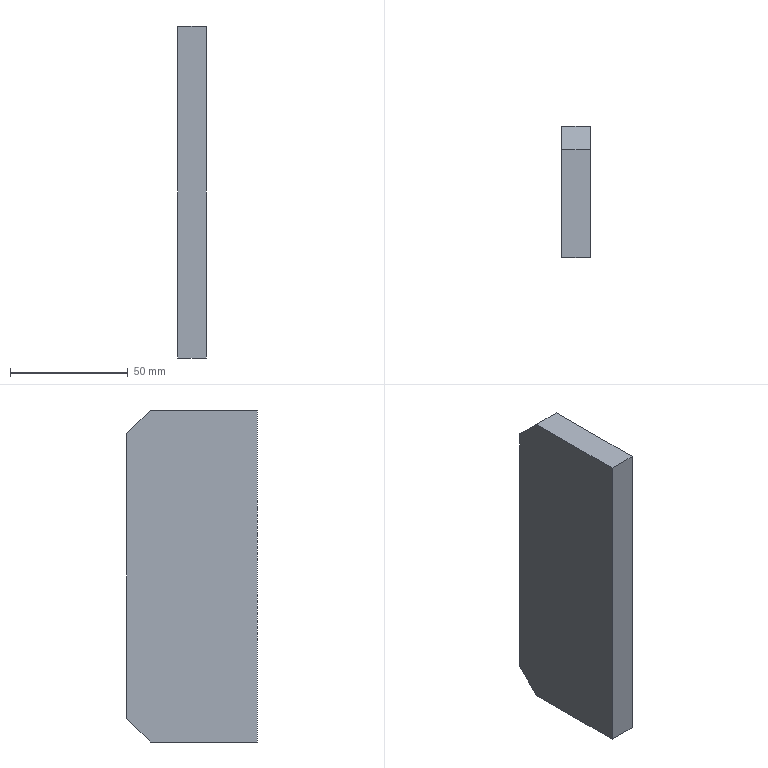Part | STEP file | RIB.1.stp | 1 solid | 8 faces | box 12 x 55.5 x 141 mm | volume 92706 mm3 | plane 8
STEP:
#1=CARTESIAN_POINT('',(0.,0.,0.));
#2=DIRECTION('',(0.,0.,1.));
#3=DIRECTION('',(1.,0.,0.));
#4=AXIS2_PLACEMENT_3D('',#1,#2,#3);
#5=CARTESIAN_POINT('',(6.,-27.75,-70.5));
#6=VERTEX_POINT('',#5);
#7=CARTESIAN_POINT('',(6.,17.75,-70.5));
#8=VERTEX_POINT('',#7);
#9=CARTESIAN_POINT('',(6.,-27.75,-70.5));
#10=DIRECTION('',(0.,1.,0.));
#11=VECTOR('',#10,1.);
#12=LINE('',#9,#11);
#13=CARTESIAN_POINT('',(6.,-0.9613,0.));
#14=DIRECTION('',(1.,0.,0.));
#15=DIRECTION('',(0.,1.,0.));
#16=AXIS2_PLACEMENT_3D('',#13,#14,#15);
#17=PLANE('',#16);
#18=CARTESIAN_POINT('',(-26.789,-70.5));
#19=DIRECTION('',(1.,0.));
#20=VECTOR('',#19,1.);
#21=LINE('',#18,#20);
#22=(GEOMETRIC_REPRESENTATION_CONTEXT(2)PARAMETRIC_REPRESENTATION_CONTEXT()REPRESENTATION_CONTEXT('',''));
#23=DEFINITIONAL_REPRESENTATION('',(#21),#22);
#24=PCURVE('',#17,#23);
#25=CARTESIAN_POINT('',(6.,-27.75,-70.5));
#26=DIRECTION('',(0.,0.,-1.));
#27=DIRECTION('',(0.,-1.,0.));
#28=AXIS2_PLACEMENT_3D('',#25,#26,#27);
#29=PLANE('',#28);
#30=CARTESIAN_POINT('',(0.,0.));
#31=DIRECTION('',(-1.,0.));
#32=VECTOR('',#31,1.);
#33=LINE('',#30,#32);
#34=(GEOMETRIC_REPRESENTATION_CONTEXT(2)PARAMETRIC_REPRESENTATION_CONTEXT()REPRESENTATION_CONTEXT('',''));
#35=DEFINITIONAL_REPRESENTATION('',(#33),#34);
#36=PCURVE('',#29,#35);
#37=SURFACE_CURVE('',#12,(#24,#36),.PCURVE_S1.);
#38=EDGE_CURVE('',#6,#8,#37,.T.);
#39=ORIENTED_EDGE('',*,*,#38,.T.);
#40=CARTESIAN_POINT('',(6.,27.75,-60.5));
#41=VERTEX_POINT('',#40);
#42=CARTESIAN_POINT('',(6.,17.75,-70.5));
#43=DIRECTION('',(0.,0.7071,0.7071));
#44=VECTOR('',#43,1.);
#45=LINE('',#42,#44);
#46=CARTESIAN_POINT('',(18.711,-70.5));
#47=DIRECTION('',(0.7071,0.7071));
#48=VECTOR('',#47,1.);
#49=LINE('',#46,#48);
#50=(GEOMETRIC_REPRESENTATION_CONTEXT(2)PARAMETRIC_REPRESENTATION_CONTEXT()REPRESENTATION_CONTEXT('',''));
#51=DEFINITIONAL_REPRESENTATION('',(#49),#50);
#52=PCURVE('',#17,#51);
#53=CARTESIAN_POINT('',(6.,17.75,-70.5));
#54=DIRECTION('',(0.,0.7071,-0.7071));
#55=DIRECTION('',(-1.,0.,0.));
#56=AXIS2_PLACEMENT_3D('',#53,#54,#55);
#57=PLANE('',#56);
#58=CARTESIAN_POINT('',(0.,0.));
#59=DIRECTION('',(0.,1.));
#60=VECTOR('',#59,1.);
#61=LINE('',#58,#60);
#62=(GEOMETRIC_REPRESENTATION_CONTEXT(2)PARAMETRIC_REPRESENTATION_CONTEXT()REPRESENTATION_CONTEXT('',''));
#63=DEFINITIONAL_REPRESENTATION('',(#61),#62);
#64=PCURVE('',#57,#63);
#65=SURFACE_CURVE('',#45,(#52,#64),.PCURVE_S1.);
#66=EDGE_CURVE('',#8,#41,#65,.T.);
#67=ORIENTED_EDGE('',*,*,#66,.T.);
#68=CARTESIAN_POINT('',(6.,27.75,60.5));
#69=VERTEX_POINT('',#68);
#70=CARTESIAN_POINT('',(6.,27.75,-60.5));
#71=DIRECTION('',(0.,0.,1.));
#72=VECTOR('',#71,1.);
#73=LINE('',#70,#72);
#74=CARTESIAN_POINT('',(28.711,-60.5));
#75=DIRECTION('',(0.,1.));
#76=VECTOR('',#75,1.);
#77=LINE('',#74,#76);
#78=(GEOMETRIC_REPRESENTATION_CONTEXT(2)PARAMETRIC_REPRESENTATION_CONTEXT()REPRESENTATION_CONTEXT('',''));
#79=DEFINITIONAL_REPRESENTATION('',(#77),#78);
#80=PCURVE('',#17,#79);
#81=CARTESIAN_POINT('',(6.,27.75,-60.5));
#82=DIRECTION('',(0.,1.,0.));
#83=DIRECTION('',(1.,0.,0.));
#84=AXIS2_PLACEMENT_3D('',#81,#82,#83);
#85=PLANE('',#84);
#86=CARTESIAN_POINT('',(0.,0.));
#87=DIRECTION('',(0.,-1.));
#88=VECTOR('',#87,1.);
#89=LINE('',#86,#88);
#90=(GEOMETRIC_REPRESENTATION_CONTEXT(2)PARAMETRIC_REPRESENTATION_CONTEXT()REPRESENTATION_CONTEXT('',''));
#91=DEFINITIONAL_REPRESENTATION('',(#89),#90);
#92=PCURVE('',#85,#91);
#93=SURFACE_CURVE('',#73,(#80,#92),.PCURVE_S1.);
#94=EDGE_CURVE('',#41,#69,#93,.T.);
#95=ORIENTED_EDGE('',*,*,#94,.T.);
#96=CARTESIAN_POINT('',(6.,17.75,70.5));
#97=VERTEX_POINT('',#96);
#98=CARTESIAN_POINT('',(6.,27.75,60.5));
#99=DIRECTION('',(0.,-0.7071,0.7071));
#100=VECTOR('',#99,1.);
#101=LINE('',#98,#100);
#102=CARTESIAN_POINT('',(28.711,60.5));
#103=DIRECTION('',(-0.7071,0.7071));
#104=VECTOR('',#103,1.);
#105=LINE('',#102,#104);
#106=(GEOMETRIC_REPRESENTATION_CONTEXT(2)PARAMETRIC_REPRESENTATION_CONTEXT()REPRESENTATION_CONTEXT('',''));
#107=DEFINITIONAL_REPRESENTATION('',(#105),#106);
#108=PCURVE('',#17,#107);
#109=CARTESIAN_POINT('',(6.,27.75,60.5));
#110=DIRECTION('',(0.,0.7071,0.7071));
#111=DIRECTION('',(1.,0.,0.));
#112=AXIS2_PLACEMENT_3D('',#109,#110,#111);
#113=PLANE('',#112);
#114=CARTESIAN_POINT('',(0.,0.));
#115=DIRECTION('',(0.,-1.));
#116=VECTOR('',#115,1.);
#117=LINE('',#114,#116);
#118=(GEOMETRIC_REPRESENTATION_CONTEXT(2)PARAMETRIC_REPRESENTATION_CONTEXT()REPRESENTATION_CONTEXT('',''));
#119=DEFINITIONAL_REPRESENTATION('',(#117),#118);
#120=PCURVE('',#113,#119);
#121=SURFACE_CURVE('',#101,(#108,#120),.PCURVE_S1.);
#122=EDGE_CURVE('',#69,#97,#121,.T.);
#123=ORIENTED_EDGE('',*,*,#122,.T.);
#124=CARTESIAN_POINT('',(6.,-27.75,70.5));
#125=VERTEX_POINT('',#124);
#126=CARTESIAN_POINT('',(6.,17.75,70.5));
#127=DIRECTION('',(0.,-1.,0.));
#128=VECTOR('',#127,1.);
#129=LINE('',#126,#128);
#130=CARTESIAN_POINT('',(18.711,70.5));
#131=DIRECTION('',(-1.,0.));
#132=VECTOR('',#131,1.);
#133=LINE('',#130,#132);
#134=(GEOMETRIC_REPRESENTATION_CONTEXT(2)PARAMETRIC_REPRESENTATION_CONTEXT()REPRESENTATION_CONTEXT('',''));
#135=DEFINITIONAL_REPRESENTATION('',(#133),#134);
#136=PCURVE('',#17,#135);
#137=CARTESIAN_POINT('',(6.,17.75,70.5));
#138=DIRECTION('',(0.,0.,1.));
#139=DIRECTION('',(1.,0.,0.));
#140=AXIS2_PLACEMENT_3D('',#137,#138,#139);
#141=PLANE('',#140);
#142=CARTESIAN_POINT('',(0.,0.));
#143=DIRECTION('',(0.,-1.));
#144=VECTOR('',#143,1.);
#145=LINE('',#142,#144);
#146=(GEOMETRIC_REPRESENTATION_CONTEXT(2)PARAMETRIC_REPRESENTATION_CONTEXT()REPRESENTATION_CONTEXT('',''));
#147=DEFINITIONAL_REPRESENTATION('',(#145),#146);
#148=PCURVE('',#141,#147);
#149=SURFACE_CURVE('',#129,(#136,#148),.PCURVE_S1.);
#150=EDGE_CURVE('',#97,#125,#149,.T.);
#151=ORIENTED_EDGE('',*,*,#150,.T.);
#152=CARTESIAN_POINT('',(6.,-27.75,-70.5));
#153=DIRECTION('',(0.,0.,1.));
#154=VECTOR('',#153,1.);
#155=LINE('',#152,#154);
#156=CARTESIAN_POINT('',(-26.789,-70.5));
#157=DIRECTION('',(0.,1.));
#158=VECTOR('',#157,1.);
#159=LINE('',#156,#158);
#160=(GEOMETRIC_REPRESENTATION_CONTEXT(2)PARAMETRIC_REPRESENTATION_CONTEXT()REPRESENTATION_CONTEXT('',''));
#161=DEFINITIONAL_REPRESENTATION('',(#159),#160);
#162=PCURVE('',#17,#161);
#163=CARTESIAN_POINT('',(6.,-27.75,70.5));
#164=DIRECTION('',(0.,-1.,0.));
#165=DIRECTION('',(0.,0.,-1.));
#166=AXIS2_PLACEMENT_3D('',#163,#164,#165);
#167=PLANE('',#166);
#168=CARTESIAN_POINT('',(141.,0.));
#169=DIRECTION('',(-1.,0.));
#170=VECTOR('',#169,1.);
#171=LINE('',#168,#170);
#172=(GEOMETRIC_REPRESENTATION_CONTEXT(2)PARAMETRIC_REPRESENTATION_CONTEXT()REPRESENTATION_CONTEXT('',''));
#173=DEFINITIONAL_REPRESENTATION('',(#171),#172);
#174=PCURVE('',#167,#173);
#175=SURFACE_CURVE('',#155,(#162,#174),.PCURVE_S1.);
#176=EDGE_CURVE('',#6,#125,#175,.T.);
#177=ORIENTED_EDGE('',*,*,#176,.F.);
#178=EDGE_LOOP('',(#39,#67,#95,#123,#151,#177));
#179=FACE_BOUND('',#178,.T.);
#180=ADVANCED_FACE('',(#179),#17,.T.);
#181=CARTESIAN_POINT('',(-6.,17.75,-70.5));
#182=VERTEX_POINT('',#181);
#183=CARTESIAN_POINT('',(-6.,27.75,-60.5));
#184=VERTEX_POINT('',#183);
#185=CARTESIAN_POINT('',(-6.,17.75,-70.5));
#186=DIRECTION('',(0.,0.7071,0.7071));
#187=VECTOR('',#186,1.);
#188=LINE('',#185,#187);
#189=CARTESIAN_POINT('',(-6.,-0.9613,0.));
#190=DIRECTION('',(1.,0.,0.));
#191=DIRECTION('',(0.,1.,0.));
#192=AXIS2_PLACEMENT_3D('',#189,#190,#191);
#193=PLANE('',#192);
#194=CARTESIAN_POINT('',(18.711,-70.5));
#195=DIRECTION('',(0.7071,0.7071));
#196=VECTOR('',#195,1.);
#197=LINE('',#194,#196);
#198=(GEOMETRIC_REPRESENTATION_CONTEXT(2)PARAMETRIC_REPRESENTATION_CONTEXT()REPRESENTATION_CONTEXT('',''));
#199=DEFINITIONAL_REPRESENTATION('',(#197),#198);
#200=PCURVE('',#193,#199);
#201=CARTESIAN_POINT('',(12.,0.));
#202=DIRECTION('',(0.,1.));
#203=VECTOR('',#202,1.);
#204=LINE('',#201,#203);
#205=(GEOMETRIC_REPRESENTATION_CONTEXT(2)PARAMETRIC_REPRESENTATION_CONTEXT()REPRESENTATION_CONTEXT('',''));
#206=DEFINITIONAL_REPRESENTATION('',(#204),#205);
#207=PCURVE('',#57,#206);
#208=SURFACE_CURVE('',#188,(#200,#207),.PCURVE_S1.);
#209=EDGE_CURVE('',#182,#184,#208,.T.);
#210=ORIENTED_EDGE('',*,*,#209,.F.);
#211=CARTESIAN_POINT('',(-6.,-27.75,-70.5));
#212=VERTEX_POINT('',#211);
#213=CARTESIAN_POINT('',(-6.,-27.75,-70.5));
#214=DIRECTION('',(0.,1.,0.));
#215=VECTOR('',#214,1.);
#216=LINE('',#213,#215);
#217=CARTESIAN_POINT('',(-26.789,-70.5));
#218=DIRECTION('',(1.,0.));
#219=VECTOR('',#218,1.);
#220=LINE('',#217,#219);
#221=(GEOMETRIC_REPRESENTATION_CONTEXT(2)PARAMETRIC_REPRESENTATION_CONTEXT()REPRESENTATION_CONTEXT('',''));
#222=DEFINITIONAL_REPRESENTATION('',(#220),#221);
#223=PCURVE('',#193,#222);
#224=CARTESIAN_POINT('',(0.,12.));
#225=DIRECTION('',(-1.,0.));
#226=VECTOR('',#225,1.);
#227=LINE('',#224,#226);
#228=(GEOMETRIC_REPRESENTATION_CONTEXT(2)PARAMETRIC_REPRESENTATION_CONTEXT()REPRESENTATION_CONTEXT('',''));
#229=DEFINITIONAL_REPRESENTATION('',(#227),#228);
#230=PCURVE('',#29,#229);
#231=SURFACE_CURVE('',#216,(#223,#230),.PCURVE_S1.);
#232=EDGE_CURVE('',#212,#182,#231,.T.);
#233=ORIENTED_EDGE('',*,*,#232,.F.);
#234=CARTESIAN_POINT('',(-6.,-27.75,70.5));
#235=VERTEX_POINT('',#234);
#236=CARTESIAN_POINT('',(-6.,-27.75,70.5));
#237=DIRECTION('',(0.,0.,-1.));
#238=VECTOR('',#237,1.);
#239=LINE('',#236,#238);
#240=CARTESIAN_POINT('',(-26.789,70.5));
#241=DIRECTION('',(0.,-1.));
#242=VECTOR('',#241,1.);
#243=LINE('',#240,#242);
#244=(GEOMETRIC_REPRESENTATION_CONTEXT(2)PARAMETRIC_REPRESENTATION_CONTEXT()REPRESENTATION_CONTEXT('',''));
#245=DEFINITIONAL_REPRESENTATION('',(#243),#244);
#246=PCURVE('',#193,#245);
#247=CARTESIAN_POINT('',(0.,-12.));
#248=DIRECTION('',(1.,0.));
#249=VECTOR('',#248,1.);
#250=LINE('',#247,#249);
#251=(GEOMETRIC_REPRESENTATION_CONTEXT(2)PARAMETRIC_REPRESENTATION_CONTEXT()REPRESENTATION_CONTEXT('',''));
#252=DEFINITIONAL_REPRESENTATION('',(#250),#251);
#253=PCURVE('',#167,#252);
#254=SURFACE_CURVE('',#239,(#246,#253),.PCURVE_S1.);
#255=EDGE_CURVE('',#235,#212,#254,.T.);
#256=ORIENTED_EDGE('',*,*,#255,.F.);
#257=CARTESIAN_POINT('',(-6.,17.75,70.5));
#258=VERTEX_POINT('',#257);
#259=CARTESIAN_POINT('',(-6.,17.75,70.5));
#260=DIRECTION('',(0.,-1.,0.));
#261=VECTOR('',#260,1.);
#262=LINE('',#259,#261);
#263=CARTESIAN_POINT('',(18.711,70.5));
#264=DIRECTION('',(-1.,0.));
#265=VECTOR('',#264,1.);
#266=LINE('',#263,#265);
#267=(GEOMETRIC_REPRESENTATION_CONTEXT(2)PARAMETRIC_REPRESENTATION_CONTEXT()REPRESENTATION_CONTEXT('',''));
#268=DEFINITIONAL_REPRESENTATION('',(#266),#267);
#269=PCURVE('',#193,#268);
#270=CARTESIAN_POINT('',(-12.,0.));
#271=DIRECTION('',(0.,-1.));
#272=VECTOR('',#271,1.);
#273=LINE('',#270,#272);
#274=(GEOMETRIC_REPRESENTATION_CONTEXT(2)PARAMETRIC_REPRESENTATION_CONTEXT()REPRESENTATION_CONTEXT('',''));
#275=DEFINITIONAL_REPRESENTATION('',(#273),#274);
#276=PCURVE('',#141,#275);
#277=SURFACE_CURVE('',#262,(#269,#276),.PCURVE_S1.);
#278=EDGE_CURVE('',#258,#235,#277,.T.);
#279=ORIENTED_EDGE('',*,*,#278,.F.);
#280=CARTESIAN_POINT('',(-6.,27.75,60.5));
#281=VERTEX_POINT('',#280);
#282=CARTESIAN_POINT('',(-6.,27.75,60.5));
#283=DIRECTION('',(0.,-0.7071,0.7071));
#284=VECTOR('',#283,1.);
#285=LINE('',#282,#284);
#286=CARTESIAN_POINT('',(28.711,60.5));
#287=DIRECTION('',(-0.7071,0.7071));
#288=VECTOR('',#287,1.);
#289=LINE('',#286,#288);
#290=(GEOMETRIC_REPRESENTATION_CONTEXT(2)PARAMETRIC_REPRESENTATION_CONTEXT()REPRESENTATION_CONTEXT('',''));
#291=DEFINITIONAL_REPRESENTATION('',(#289),#290);
#292=PCURVE('',#193,#291);
#293=CARTESIAN_POINT('',(-12.,0.));
#294=DIRECTION('',(0.,-1.));
#295=VECTOR('',#294,1.);
#296=LINE('',#293,#295);
#297=(GEOMETRIC_REPRESENTATION_CONTEXT(2)PARAMETRIC_REPRESENTATION_CONTEXT()REPRESENTATION_CONTEXT('',''));
#298=DEFINITIONAL_REPRESENTATION('',(#296),#297);
#299=PCURVE('',#113,#298);
#300=SURFACE_CURVE('',#285,(#292,#299),.PCURVE_S1.);
#301=EDGE_CURVE('',#281,#258,#300,.T.);
#302=ORIENTED_EDGE('',*,*,#301,.F.);
#303=CARTESIAN_POINT('',(-6.,27.75,-60.5));
#304=DIRECTION('',(0.,0.,1.));
#305=VECTOR('',#304,1.);
#306=LINE('',#303,#305);
#307=CARTESIAN_POINT('',(28.711,-60.5));
#308=DIRECTION('',(0.,1.));
#309=VECTOR('',#308,1.);
#310=LINE('',#307,#309);
#311=(GEOMETRIC_REPRESENTATION_CONTEXT(2)PARAMETRIC_REPRESENTATION_CONTEXT()REPRESENTATION_CONTEXT('',''));
#312=DEFINITIONAL_REPRESENTATION('',(#310),#311);
#313=PCURVE('',#193,#312);
#314=CARTESIAN_POINT('',(-12.,0.));
#315=DIRECTION('',(0.,-1.));
#316=VECTOR('',#315,1.);
#317=LINE('',#314,#316);
#318=(GEOMETRIC_REPRESENTATION_CONTEXT(2)PARAMETRIC_REPRESENTATION_CONTEXT()REPRESENTATION_CONTEXT('',''));
#319=DEFINITIONAL_REPRESENTATION('',(#317),#318);
#320=PCURVE('',#85,#319);
#321=SURFACE_CURVE('',#306,(#313,#320),.PCURVE_S1.);
#322=EDGE_CURVE('',#184,#281,#321,.T.);
#323=ORIENTED_EDGE('',*,*,#322,.F.);
#324=EDGE_LOOP('',(#210,#233,#256,#279,#302,#323));
#325=FACE_BOUND('',#324,.T.);
#326=ADVANCED_FACE('',(#325),#193,.F.);
#327=ORIENTED_EDGE('',*,*,#232,.T.);
#328=CARTESIAN_POINT('',(6.,17.75,-70.5));
#329=DIRECTION('',(-1.,0.,0.));
#330=VECTOR('',#329,1.);
#331=LINE('',#328,#330);
#332=CARTESIAN_POINT('',(-45.5,0.));
#333=DIRECTION('',(0.,1.));
#334=VECTOR('',#333,1.);
#335=LINE('',#332,#334);
#336=(GEOMETRIC_REPRESENTATION_CONTEXT(2)PARAMETRIC_REPRESENTATION_CONTEXT()REPRESENTATION_CONTEXT('',''));
#337=DEFINITIONAL_REPRESENTATION('',(#335),#336);
#338=PCURVE('',#29,#337);
#339=CARTESIAN_POINT('',(0.,0.));
#340=DIRECTION('',(1.,0.));
#341=VECTOR('',#340,1.);
#342=LINE('',#339,#341);
#343=(GEOMETRIC_REPRESENTATION_CONTEXT(2)PARAMETRIC_REPRESENTATION_CONTEXT()REPRESENTATION_CONTEXT('',''));
#344=DEFINITIONAL_REPRESENTATION('',(#342),#343);
#345=PCURVE('',#57,#344);
#346=SURFACE_CURVE('',#331,(#338,#345),.PCURVE_S1.);
#347=EDGE_CURVE('',#8,#182,#346,.T.);
#348=ORIENTED_EDGE('',*,*,#347,.F.);
#349=ORIENTED_EDGE('',*,*,#38,.F.);
#350=CARTESIAN_POINT('',(6.,-27.75,-70.5));
#351=DIRECTION('',(-1.,0.,0.));
#352=VECTOR('',#351,1.);
#353=LINE('',#350,#352);
#354=CARTESIAN_POINT('',(0.,0.));
#355=DIRECTION('',(0.,1.));
#356=VECTOR('',#355,1.);
#357=LINE('',#354,#356);
#358=(GEOMETRIC_REPRESENTATION_CONTEXT(2)PARAMETRIC_REPRESENTATION_CONTEXT()REPRESENTATION_CONTEXT('',''));
#359=DEFINITIONAL_REPRESENTATION('',(#357),#358);
#360=PCURVE('',#29,#359);
#361=CARTESIAN_POINT('',(141.,0.));
#362=DIRECTION('',(0.,-1.));
#363=VECTOR('',#362,1.);
#364=LINE('',#361,#363);
#365=(GEOMETRIC_REPRESENTATION_CONTEXT(2)PARAMETRIC_REPRESENTATION_CONTEXT()REPRESENTATION_CONTEXT('',''));
#366=DEFINITIONAL_REPRESENTATION('',(#364),#365);
#367=PCURVE('',#167,#366);
#368=SURFACE_CURVE('',#353,(#360,#367),.PCURVE_S1.);
#369=EDGE_CURVE('',#6,#212,#368,.T.);
#370=ORIENTED_EDGE('',*,*,#369,.T.);
#371=EDGE_LOOP('',(#327,#348,#349,#370));
#372=FACE_BOUND('',#371,.T.);
#373=ADVANCED_FACE('',(#372),#29,.T.);
#374=ORIENTED_EDGE('',*,*,#255,.T.);
#375=ORIENTED_EDGE('',*,*,#369,.F.);
#376=ORIENTED_EDGE('',*,*,#176,.T.);
#377=CARTESIAN_POINT('',(6.,-27.75,70.5));
#378=DIRECTION('',(-1.,0.,0.));
#379=VECTOR('',#378,1.);
#380=LINE('',#377,#379);
#381=CARTESIAN_POINT('',(0.,0.));
#382=DIRECTION('',(0.,-1.));
#383=VECTOR('',#382,1.);
#384=LINE('',#381,#383);
#385=(GEOMETRIC_REPRESENTATION_CONTEXT(2)PARAMETRIC_REPRESENTATION_CONTEXT()REPRESENTATION_CONTEXT('',''));
#386=DEFINITIONAL_REPRESENTATION('',(#384),#385);
#387=PCURVE('',#167,#386);
#388=CARTESIAN_POINT('',(0.,-45.5));
#389=DIRECTION('',(-1.,0.));
#390=VECTOR('',#389,1.);
#391=LINE('',#388,#390);
#392=(GEOMETRIC_REPRESENTATION_CONTEXT(2)PARAMETRIC_REPRESENTATION_CONTEXT()REPRESENTATION_CONTEXT('',''));
#393=DEFINITIONAL_REPRESENTATION('',(#391),#392);
#394=PCURVE('',#141,#393);
#395=SURFACE_CURVE('',#380,(#387,#394),.PCURVE_S1.);
#396=EDGE_CURVE('',#125,#235,#395,.T.);
#397=ORIENTED_EDGE('',*,*,#396,.T.);
#398=EDGE_LOOP('',(#374,#375,#376,#397));
#399=FACE_BOUND('',#398,.T.);
#400=ADVANCED_FACE('',(#399),#167,.T.);
#401=ORIENTED_EDGE('',*,*,#278,.T.);
#402=ORIENTED_EDGE('',*,*,#396,.F.);
#403=ORIENTED_EDGE('',*,*,#150,.F.);
#404=CARTESIAN_POINT('',(6.,17.75,70.5));
#405=DIRECTION('',(-1.,0.,0.));
#406=VECTOR('',#405,1.);
#407=LINE('',#404,#406);
#408=CARTESIAN_POINT('',(0.,0.));
#409=DIRECTION('',(-1.,0.));
#410=VECTOR('',#409,1.);
#411=LINE('',#408,#410);
#412=(GEOMETRIC_REPRESENTATION_CONTEXT(2)PARAMETRIC_REPRESENTATION_CONTEXT()REPRESENTATION_CONTEXT('',''));
#413=DEFINITIONAL_REPRESENTATION('',(#411),#412);
#414=PCURVE('',#141,#413);
#415=CARTESIAN_POINT('',(0.,-14.142));
#416=DIRECTION('',(-1.,0.));
#417=VECTOR('',#416,1.);
#418=LINE('',#415,#417);
#419=(GEOMETRIC_REPRESENTATION_CONTEXT(2)PARAMETRIC_REPRESENTATION_CONTEXT()REPRESENTATION_CONTEXT('',''));
#420=DEFINITIONAL_REPRESENTATION('',(#418),#419);
#421=PCURVE('',#113,#420);
#422=SURFACE_CURVE('',#407,(#414,#421),.PCURVE_S1.);
#423=EDGE_CURVE('',#97,#258,#422,.T.);
#424=ORIENTED_EDGE('',*,*,#423,.T.);
#425=EDGE_LOOP('',(#401,#402,#403,#424));
#426=FACE_BOUND('',#425,.T.);
#427=ADVANCED_FACE('',(#426),#141,.T.);
#428=ORIENTED_EDGE('',*,*,#301,.T.);
#429=ORIENTED_EDGE('',*,*,#423,.F.);
#430=ORIENTED_EDGE('',*,*,#122,.F.);
#431=CARTESIAN_POINT('',(6.,27.75,60.5));
#432=DIRECTION('',(-1.,0.,0.));
#433=VECTOR('',#432,1.);
#434=LINE('',#431,#433);
#435=CARTESIAN_POINT('',(0.,0.));
#436=DIRECTION('',(-1.,0.));
#437=VECTOR('',#436,1.);
#438=LINE('',#435,#437);
#439=(GEOMETRIC_REPRESENTATION_CONTEXT(2)PARAMETRIC_REPRESENTATION_CONTEXT()REPRESENTATION_CONTEXT('',''));
#440=DEFINITIONAL_REPRESENTATION('',(#438),#439);
#441=PCURVE('',#113,#440);
#442=CARTESIAN_POINT('',(0.,-121.));
#443=DIRECTION('',(-1.,0.));
#444=VECTOR('',#443,1.);
#445=LINE('',#442,#444);
#446=(GEOMETRIC_REPRESENTATION_CONTEXT(2)PARAMETRIC_REPRESENTATION_CONTEXT()REPRESENTATION_CONTEXT('',''));
#447=DEFINITIONAL_REPRESENTATION('',(#445),#446);
#448=PCURVE('',#85,#447);
#449=SURFACE_CURVE('',#434,(#441,#448),.PCURVE_S1.);
#450=EDGE_CURVE('',#69,#281,#449,.T.);
#451=ORIENTED_EDGE('',*,*,#450,.T.);
#452=EDGE_LOOP('',(#428,#429,#430,#451));
#453=FACE_BOUND('',#452,.T.);
#454=ADVANCED_FACE('',(#453),#113,.T.);
#455=ORIENTED_EDGE('',*,*,#322,.T.);
#456=ORIENTED_EDGE('',*,*,#450,.F.);
#457=ORIENTED_EDGE('',*,*,#94,.F.);
#458=CARTESIAN_POINT('',(6.,27.75,-60.5));
#459=DIRECTION('',(-1.,0.,0.));
#460=VECTOR('',#459,1.);
#461=LINE('',#458,#460);
#462=CARTESIAN_POINT('',(0.,0.));
#463=DIRECTION('',(-1.,0.));
#464=VECTOR('',#463,1.);
#465=LINE('',#462,#464);
#466=(GEOMETRIC_REPRESENTATION_CONTEXT(2)PARAMETRIC_REPRESENTATION_CONTEXT()REPRESENTATION_CONTEXT('',''));
#467=DEFINITIONAL_REPRESENTATION('',(#465),#466);
#468=PCURVE('',#85,#467);
#469=CARTESIAN_POINT('',(0.,14.142));
#470=DIRECTION('',(1.,0.));
#471=VECTOR('',#470,1.);
#472=LINE('',#469,#471);
#473=(GEOMETRIC_REPRESENTATION_CONTEXT(2)PARAMETRIC_REPRESENTATION_CONTEXT()REPRESENTATION_CONTEXT('',''));
#474=DEFINITIONAL_REPRESENTATION('',(#472),#473);
#475=PCURVE('',#57,#474);
#476=SURFACE_CURVE('',#461,(#468,#475),.PCURVE_S1.);
#477=EDGE_CURVE('',#41,#184,#476,.T.);
#478=ORIENTED_EDGE('',*,*,#477,.T.);
#479=EDGE_LOOP('',(#455,#456,#457,#478));
#480=FACE_BOUND('',#479,.T.);
#481=ADVANCED_FACE('',(#480),#85,.T.);
#482=ORIENTED_EDGE('',*,*,#209,.T.);
#483=ORIENTED_EDGE('',*,*,#477,.F.);
#484=ORIENTED_EDGE('',*,*,#66,.F.);
#485=ORIENTED_EDGE('',*,*,#347,.T.);
#486=EDGE_LOOP('',(#482,#483,#484,#485));
#487=FACE_BOUND('',#486,.T.);
#488=ADVANCED_FACE('',(#487),#57,.T.);
#489=CLOSED_SHELL('',(#180,#326,#373,#400,#427,#454,#481,#488));
#490=MANIFOLD_SOLID_BREP('',#489);
#491=(LENGTH_UNIT()NAMED_UNIT(*)SI_UNIT(.MILLI.,.METRE.));
#492=UNCERTAINTY_MEASURE_WITH_UNIT(LENGTH_MEASURE(0.0000001),#491,'','');
#493=(NAMED_UNIT(*)PLANE_ANGLE_UNIT()SI_UNIT($,.RADIAN.));
#494=(NAMED_UNIT(*)SI_UNIT($,.STERADIAN.)SOLID_ANGLE_UNIT());
#495=(GEOMETRIC_REPRESENTATION_CONTEXT(3)GLOBAL_UNCERTAINTY_ASSIGNED_CONTEXT((#492))GLOBAL_UNIT_ASSIGNED_CONTEXT((#491,#493,#494))REPRESENTATION_CONTEXT('',''));
#496=ADVANCED_BREP_SHAPE_REPRESENTATION('',(#4,#490),#495);